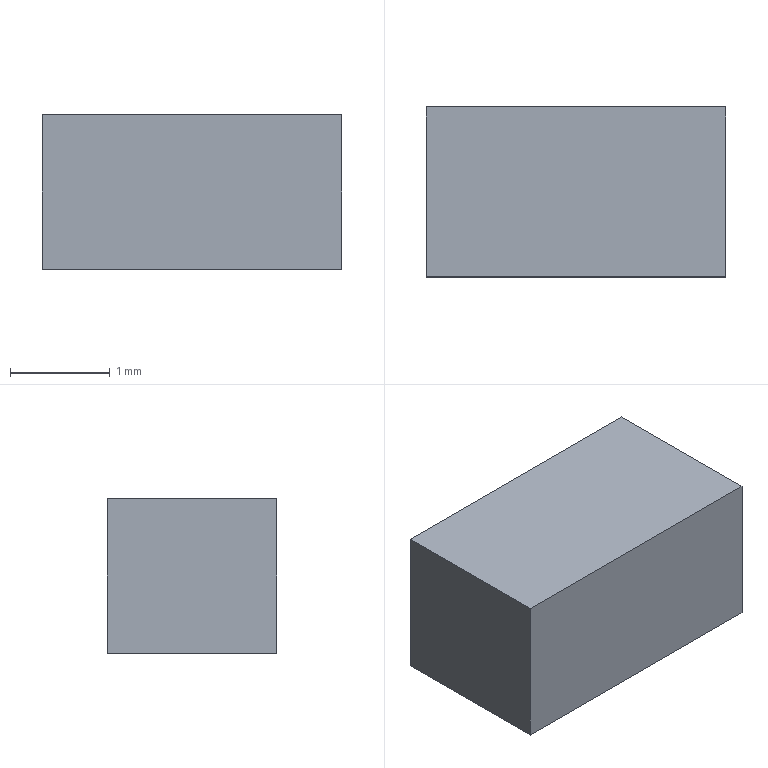Part | Creo | 1 solid | 6 faces | box 3 x 1.7 x 1.55 mm | volume 7.906 mm3 | plane 6
STEP:
#1=CARTESIAN_POINT('',(0.,0.,0.));
#2=DIRECTION('',(0.,0.,1.));
#3=DIRECTION('',(1.,0.,0.));
#4=AXIS2_PLACEMENT_3D('',#1,#2,#3);
#5=CARTESIAN_POINT('',(-1.5,-0.85,0.));
#6=VERTEX_POINT('',#5);
#7=CARTESIAN_POINT('',(1.5,-0.85,0.));
#8=VERTEX_POINT('',#7);
#9=CARTESIAN_POINT('',(-1.5,-0.85,0.));
#10=DIRECTION('',(1.,0.,0.));
#11=VECTOR('',#10,3.);
#12=LINE('',#9,#11);
#13=EDGE_CURVE('',#6,#8,#12,.T.);
#14=ORIENTED_EDGE('',*,*,#13,.T.);
#15=CARTESIAN_POINT('',(1.5,0.85,0.));
#16=VERTEX_POINT('',#15);
#17=CARTESIAN_POINT('',(1.5,-0.85,0.));
#18=DIRECTION('',(0.,1.,0.));
#19=VECTOR('',#18,1.7);
#20=LINE('',#17,#19);
#21=EDGE_CURVE('',#8,#16,#20,.T.);
#22=ORIENTED_EDGE('',*,*,#21,.T.);
#23=CARTESIAN_POINT('',(-1.5,0.85,0.));
#24=VERTEX_POINT('',#23);
#25=CARTESIAN_POINT('',(1.5,0.85,0.));
#26=DIRECTION('',(-1.,0.,0.));
#27=VECTOR('',#26,3.);
#28=LINE('',#25,#27);
#29=EDGE_CURVE('',#16,#24,#28,.T.);
#30=ORIENTED_EDGE('',*,*,#29,.T.);
#31=CARTESIAN_POINT('',(-1.5,0.85,0.));
#32=DIRECTION('',(0.,-1.,0.));
#33=VECTOR('',#32,1.7);
#34=LINE('',#31,#33);
#35=EDGE_CURVE('',#24,#6,#34,.T.);
#36=ORIENTED_EDGE('',*,*,#35,.T.);
#37=EDGE_LOOP('',(#14,#22,#30,#36));
#38=FACE_OUTER_BOUND('',#37,.F.);
#39=CARTESIAN_POINT('',(0.,0.,0.));
#40=DIRECTION('',(0.,0.,1.));
#41=DIRECTION('',(1.,0.,0.));
#42=AXIS2_PLACEMENT_3D('',#39,#40,#41);
#43=PLANE('',#42);
#44=ADVANCED_FACE('',(#38),#43,.F.);
#45=ORIENTED_EDGE('',*,*,#13,.F.);
#46=CARTESIAN_POINT('',(-1.5,-0.85,1.55));
#47=VERTEX_POINT('',#46);
#48=CARTESIAN_POINT('',(-1.5,-0.85,0.));
#49=DIRECTION('',(0.,0.,1.));
#50=VECTOR('',#49,1.55);
#51=LINE('',#48,#50);
#52=EDGE_CURVE('',#6,#47,#51,.T.);
#53=ORIENTED_EDGE('',*,*,#52,.T.);
#54=CARTESIAN_POINT('',(1.5,-0.85,1.55));
#55=VERTEX_POINT('',#54);
#56=CARTESIAN_POINT('',(-1.5,-0.85,1.55));
#57=DIRECTION('',(1.,0.,0.));
#58=VECTOR('',#57,3.);
#59=LINE('',#56,#58);
#60=EDGE_CURVE('',#47,#55,#59,.T.);
#61=ORIENTED_EDGE('',*,*,#60,.T.);
#62=CARTESIAN_POINT('',(1.5,-0.85,0.));
#63=DIRECTION('',(0.,0.,1.));
#64=VECTOR('',#63,1.55);
#65=LINE('',#62,#64);
#66=EDGE_CURVE('',#8,#55,#65,.T.);
#67=ORIENTED_EDGE('',*,*,#66,.F.);
#68=EDGE_LOOP('',(#45,#53,#61,#67));
#69=FACE_OUTER_BOUND('',#68,.F.);
#70=CARTESIAN_POINT('',(-1.5,-0.85,0.));
#71=DIRECTION('',(0.,-1.,0.));
#72=DIRECTION('',(1.,0.,0.));
#73=AXIS2_PLACEMENT_3D('',#70,#71,#72);
#74=PLANE('',#73);
#75=ADVANCED_FACE('',(#69),#74,.T.);
#76=ORIENTED_EDGE('',*,*,#35,.F.);
#77=CARTESIAN_POINT('',(-1.5,0.85,1.55));
#78=VERTEX_POINT('',#77);
#79=CARTESIAN_POINT('',(-1.5,0.85,0.));
#80=DIRECTION('',(0.,0.,1.));
#81=VECTOR('',#80,1.55);
#82=LINE('',#79,#81);
#83=EDGE_CURVE('',#24,#78,#82,.T.);
#84=ORIENTED_EDGE('',*,*,#83,.T.);
#85=CARTESIAN_POINT('',(-1.5,0.85,1.55));
#86=DIRECTION('',(0.,-1.,0.));
#87=VECTOR('',#86,1.7);
#88=LINE('',#85,#87);
#89=EDGE_CURVE('',#78,#47,#88,.T.);
#90=ORIENTED_EDGE('',*,*,#89,.T.);
#91=ORIENTED_EDGE('',*,*,#52,.F.);
#92=EDGE_LOOP('',(#76,#84,#90,#91));
#93=FACE_OUTER_BOUND('',#92,.F.);
#94=CARTESIAN_POINT('',(-1.5,0.85,0.));
#95=DIRECTION('',(-1.,0.,0.));
#96=DIRECTION('',(0.,-1.,0.));
#97=AXIS2_PLACEMENT_3D('',#94,#95,#96);
#98=PLANE('',#97);
#99=ADVANCED_FACE('',(#93),#98,.T.);
#100=ORIENTED_EDGE('',*,*,#29,.F.);
#101=CARTESIAN_POINT('',(1.5,0.85,1.55));
#102=VERTEX_POINT('',#101);
#103=CARTESIAN_POINT('',(1.5,0.85,0.));
#104=DIRECTION('',(0.,0.,1.));
#105=VECTOR('',#104,1.55);
#106=LINE('',#103,#105);
#107=EDGE_CURVE('',#16,#102,#106,.T.);
#108=ORIENTED_EDGE('',*,*,#107,.T.);
#109=CARTESIAN_POINT('',(1.5,0.85,1.55));
#110=DIRECTION('',(-1.,0.,0.));
#111=VECTOR('',#110,3.);
#112=LINE('',#109,#111);
#113=EDGE_CURVE('',#102,#78,#112,.T.);
#114=ORIENTED_EDGE('',*,*,#113,.T.);
#115=ORIENTED_EDGE('',*,*,#83,.F.);
#116=EDGE_LOOP('',(#100,#108,#114,#115));
#117=FACE_OUTER_BOUND('',#116,.F.);
#118=CARTESIAN_POINT('',(1.5,0.85,0.));
#119=DIRECTION('',(0.,1.,0.));
#120=DIRECTION('',(-1.,0.,0.));
#121=AXIS2_PLACEMENT_3D('',#118,#119,#120);
#122=PLANE('',#121);
#123=ADVANCED_FACE('',(#117),#122,.T.);
#124=ORIENTED_EDGE('',*,*,#21,.F.);
#125=ORIENTED_EDGE('',*,*,#66,.T.);
#126=CARTESIAN_POINT('',(1.5,-0.85,1.55));
#127=DIRECTION('',(0.,1.,0.));
#128=VECTOR('',#127,1.7);
#129=LINE('',#126,#128);
#130=EDGE_CURVE('',#55,#102,#129,.T.);
#131=ORIENTED_EDGE('',*,*,#130,.T.);
#132=ORIENTED_EDGE('',*,*,#107,.F.);
#133=EDGE_LOOP('',(#124,#125,#131,#132));
#134=FACE_OUTER_BOUND('',#133,.F.);
#135=CARTESIAN_POINT('',(1.5,-0.85,0.));
#136=DIRECTION('',(1.,0.,0.));
#137=DIRECTION('',(0.,1.,0.));
#138=AXIS2_PLACEMENT_3D('',#135,#136,#137);
#139=PLANE('',#138);
#140=ADVANCED_FACE('',(#134),#139,.T.);
#141=ORIENTED_EDGE('',*,*,#60,.F.);
#142=ORIENTED_EDGE('',*,*,#89,.F.);
#143=ORIENTED_EDGE('',*,*,#113,.F.);
#144=ORIENTED_EDGE('',*,*,#130,.F.);
#145=EDGE_LOOP('',(#141,#142,#143,#144));
#146=FACE_OUTER_BOUND('',#145,.F.);
#147=CARTESIAN_POINT('',(0.,0.,1.55));
#148=DIRECTION('',(0.,0.,1.));
#149=DIRECTION('',(1.,0.,0.));
#150=AXIS2_PLACEMENT_3D('',#147,#148,#149);
#151=PLANE('',#150);
#152=ADVANCED_FACE('',(#146),#151,.T.);
#153=CLOSED_SHELL('',(#44,#75,#99,#123,#140,#152));
#154=MANIFOLD_SOLID_BREP('',#153);
#155=(LENGTH_UNIT()NAMED_UNIT(*)SI_UNIT(.MILLI.,.METRE.));
#156=UNCERTAINTY_MEASURE_WITH_UNIT(LENGTH_MEASURE(0.0003781),#155,'','');
#157=(NAMED_UNIT(*)PLANE_ANGLE_UNIT()SI_UNIT($,.RADIAN.));
#158=PLANE_ANGLE_MEASURE_WITH_UNIT(PLANE_ANGLE_MEASURE(0.01745),#157);
#159=(CONVERSION_BASED_UNIT('DEGREE',#158)NAMED_UNIT(*)PLANE_ANGLE_UNIT());
#160=(NAMED_UNIT(*)SI_UNIT($,.STERADIAN.)SOLID_ANGLE_UNIT());
#161=(GEOMETRIC_REPRESENTATION_CONTEXT(3)GLOBAL_UNCERTAINTY_ASSIGNED_CONTEXT((#156))GLOBAL_UNIT_ASSIGNED_CONTEXT((#155,#159,#160))REPRESENTATION_CONTEXT('',''));
#162=ADVANCED_BREP_SHAPE_REPRESENTATION('',(#4,#154),#161);